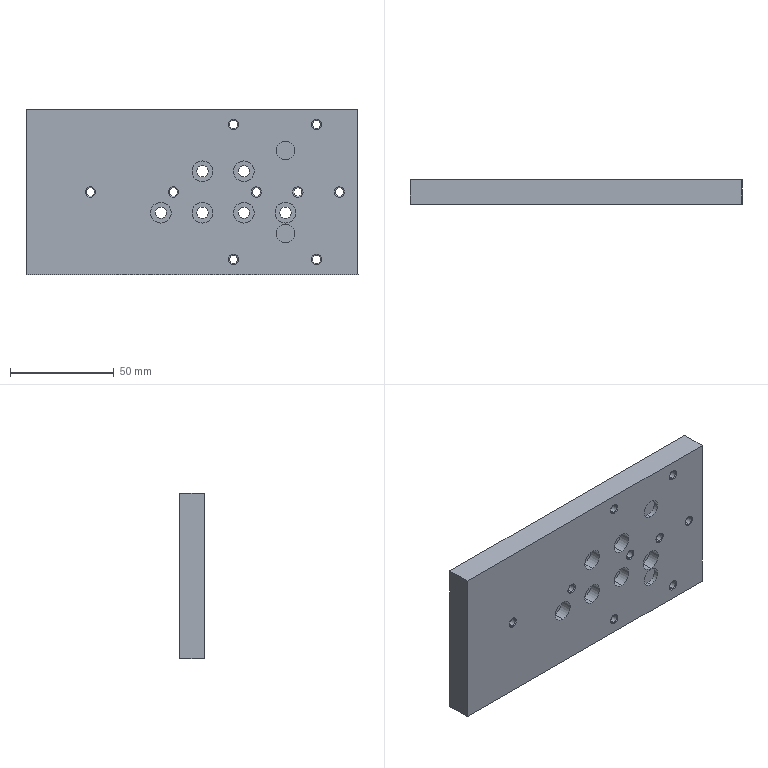Part | STEP file | 00684281_ADAPTERPLATTE_HMVY-1 | 1 solid | 127 faces | box 160 x 12 x 80 mm | volume 147813 mm3 | cylinder 58 | cone 49 | plane 20 | commonest cylinder face diameters 4.019 x18 9 x16 5.5 x12 10 x12